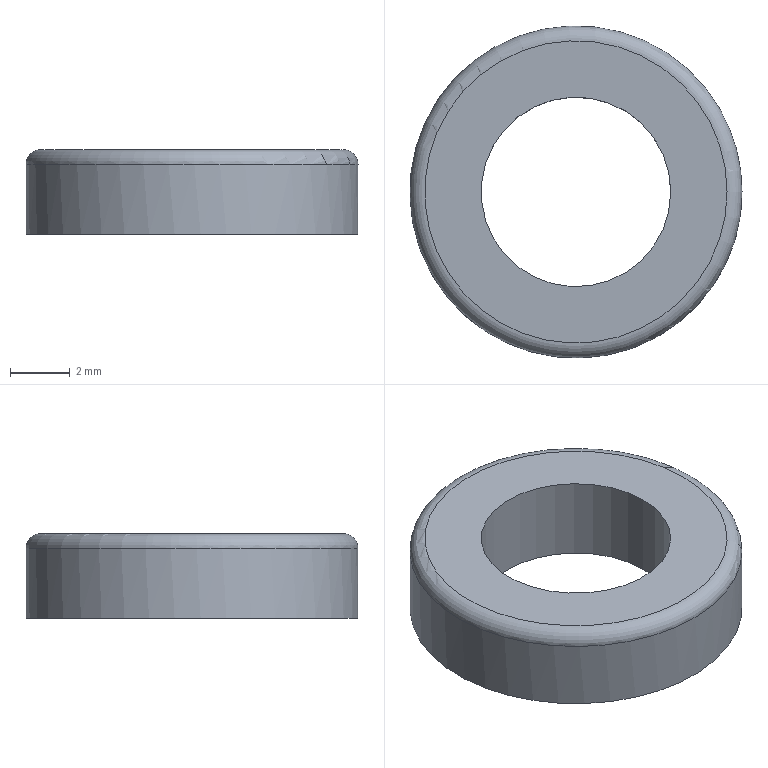Part | NX | features solid 2 | 1 solid | 5 faces | box 11.125 x 11.125 x 2.845 mm | volume 184.609 mm3 | cylinder 2 | plane 2 | torus 1 | commonest cylinder face diameters 6.35 x1 11.125 x1
STEP:
#1=CARTESIAN_POINT('',(5.563,0.,7.425));
#2=VERTEX_POINT('',#1);
#3=CARTESIAN_POINT('',(0.,0.,7.425));
#4=DIRECTION('',(0.,0.,1.));
#5=DIRECTION('',(1.,0.,0.));
#6=AXIS2_PLACEMENT_3D('',#3,#4,#5);
#7=CIRCLE('',#6,5.563);
#8=EDGE_CURVE('',#2,#2,#7,.F.);
#9=ORIENTED_EDGE('',*,*,#8,.T.);
#10=EDGE_LOOP('',(#9));
#11=FACE_BOUND('',#10,.T.);
#12=CARTESIAN_POINT('',(4.817,2.781,5.08));
#13=VERTEX_POINT('',#12);
#14=CARTESIAN_POINT('',(0.,0.,5.08));
#15=DIRECTION('',(0.,0.,1.));
#16=DIRECTION('',(0.866,0.5,0.));
#17=AXIS2_PLACEMENT_3D('',#14,#15,#16);
#18=CIRCLE('',#17,5.563);
#19=EDGE_CURVE('',#13,#13,#18,.T.);
#20=ORIENTED_EDGE('',*,*,#19,.T.);
#21=EDGE_LOOP('',(#20));
#22=FACE_BOUND('',#21,.T.);
#23=CARTESIAN_POINT('',(0.,0.,7.925));
#24=DIRECTION('',(0.,0.,-1.));
#25=DIRECTION('',(-1.,0.,0.));
#26=AXIS2_PLACEMENT_3D('',#23,#24,#25);
#27=CYLINDRICAL_SURFACE('',#26,5.563);
#28=ADVANCED_FACE('',(#11,#22),#27,.T.);
#29=CARTESIAN_POINT('',(3.175,0.,7.925));
#30=VERTEX_POINT('',#29);
#31=CARTESIAN_POINT('',(0.,0.,7.925));
#32=DIRECTION('',(0.,0.,1.));
#33=DIRECTION('',(1.,0.,0.));
#34=AXIS2_PLACEMENT_3D('',#31,#32,#33);
#35=CIRCLE('',#34,3.175);
#36=EDGE_CURVE('',#30,#30,#35,.T.);
#37=ORIENTED_EDGE('',*,*,#36,.T.);
#38=EDGE_LOOP('',(#37));
#39=FACE_BOUND('',#38,.T.);
#40=CARTESIAN_POINT('',(3.175,0.,5.08));
#41=VERTEX_POINT('',#40);
#42=CARTESIAN_POINT('',(0.,0.,5.08));
#43=DIRECTION('',(0.,0.,1.));
#44=DIRECTION('',(1.,0.,0.));
#45=AXIS2_PLACEMENT_3D('',#42,#43,#44);
#46=CIRCLE('',#45,3.175);
#47=EDGE_CURVE('',#41,#41,#46,.T.);
#48=ORIENTED_EDGE('',*,*,#47,.F.);
#49=EDGE_LOOP('',(#48));
#50=FACE_BOUND('',#49,.T.);
#51=CARTESIAN_POINT('',(0.,0.,7.925));
#52=DIRECTION('',(0.,0.,-1.));
#53=DIRECTION('',(-1.,0.,0.));
#54=AXIS2_PLACEMENT_3D('',#51,#52,#53);
#55=CYLINDRICAL_SURFACE('',#54,3.175);
#56=ADVANCED_FACE('',(#39,#50),#55,.F.);
#57=CARTESIAN_POINT('',(5.063,0.,7.925));
#58=VERTEX_POINT('',#57);
#59=CARTESIAN_POINT('',(0.,0.,7.925));
#60=DIRECTION('',(0.,0.,1.));
#61=DIRECTION('',(1.,0.,0.));
#62=AXIS2_PLACEMENT_3D('',#59,#60,#61);
#63=CIRCLE('',#62,5.063);
#64=EDGE_CURVE('',#58,#58,#63,.T.);
#65=ORIENTED_EDGE('',*,*,#64,.T.);
#66=EDGE_LOOP('',(#65));
#67=FACE_BOUND('',#66,.T.);
#68=ORIENTED_EDGE('',*,*,#36,.F.);
#69=EDGE_LOOP('',(#68));
#70=FACE_BOUND('',#69,.T.);
#71=CARTESIAN_POINT('',(0.,0.,7.925));
#72=DIRECTION('',(0.,0.,1.));
#73=DIRECTION('',(1.,0.,0.));
#74=AXIS2_PLACEMENT_3D('',#71,#72,#73);
#75=PLANE('',#74);
#76=ADVANCED_FACE('',(#67,#70),#75,.T.);
#77=ORIENTED_EDGE('',*,*,#19,.F.);
#78=EDGE_LOOP('',(#77));
#79=FACE_BOUND('',#78,.T.);
#80=ORIENTED_EDGE('',*,*,#47,.T.);
#81=EDGE_LOOP('',(#80));
#82=FACE_BOUND('',#81,.T.);
#83=CARTESIAN_POINT('',(0.,0.,5.08));
#84=DIRECTION('',(0.,0.,1.));
#85=DIRECTION('',(1.,0.,0.));
#86=AXIS2_PLACEMENT_3D('',#83,#84,#85);
#87=PLANE('',#86);
#88=ADVANCED_FACE('',(#79,#82),#87,.F.);
#89=ORIENTED_EDGE('',*,*,#8,.F.);
#90=EDGE_LOOP('',(#89));
#91=FACE_BOUND('',#90,.T.);
#92=ORIENTED_EDGE('',*,*,#64,.F.);
#93=EDGE_LOOP('',(#92));
#94=FACE_BOUND('',#93,.T.);
#95=CARTESIAN_POINT('',(0.,0.,7.425));
#96=DIRECTION('',(0.,0.,1.));
#97=DIRECTION('',(1.,0.,0.));
#98=AXIS2_PLACEMENT_3D('',#95,#96,#97);
#99=TOROIDAL_SURFACE('',#98,5.063,0.5);
#100=ADVANCED_FACE('',(#91,#94),#99,.T.);
#101=CLOSED_SHELL('',(#28,#56,#76,#88,#100));
#102=MANIFOLD_SOLID_BREP('',#101);
#103=(LENGTH_UNIT()NAMED_UNIT(*)SI_UNIT(.MILLI.,.METRE.));
#104=UNCERTAINTY_MEASURE_WITH_UNIT(LENGTH_MEASURE(0.00001),#103,'','');
#105=(NAMED_UNIT(*)PLANE_ANGLE_UNIT()SI_UNIT($,.RADIAN.));
#106=(NAMED_UNIT(*)SI_UNIT($,.STERADIAN.)SOLID_ANGLE_UNIT());
#107=(GEOMETRIC_REPRESENTATION_CONTEXT(3)GLOBAL_UNCERTAINTY_ASSIGNED_CONTEXT((#104))GLOBAL_UNIT_ASSIGNED_CONTEXT((#103,#105,#106))REPRESENTATION_CONTEXT('',''));
#108=ADVANCED_BREP_SHAPE_REPRESENTATION('',(#102),#107);